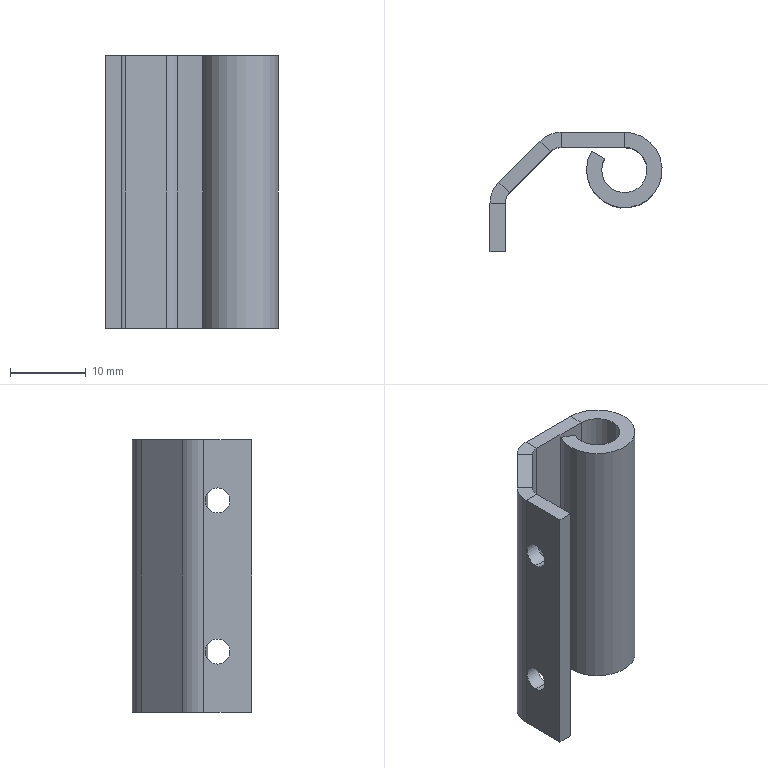Part | SolidWorks | features EdgeFlange 2, FlatPattern 1, Hem 1, HoleWzd 1, SMBaseFlange 1, SheetMetal 1 | 1 solid | 30 faces | box 22.778 x 15.778 x 36 mm | volume 3424 mm3 | plane 20 | cylinder 10 | commonest cylinder face diameters 3.3 x4 4 x2 8 x2 6 x1 10 x1
STEP:
#1=CARTESIAN_POINT('',(-12.278,-11.278,-11.65));
#2=VERTEX_POINT('',#1);
#3=CARTESIAN_POINT('',(-12.278,-11.278,-8.35));
#4=VERTEX_POINT('',#3);
#5=CARTESIAN_POINT('',(-12.278,-11.278,-10.));
#6=DIRECTION('',(-1.,0.,0.));
#7=DIRECTION('',(0.,-1.,0.));
#8=AXIS2_PLACEMENT_3D('',#5,#6,#7);
#9=CIRCLE('',#8,1.65);
#10=EDGE_CURVE('',#2,#4,#9,.T.);
#11=ORIENTED_EDGE('',*,*,#10,.F.);
#12=CARTESIAN_POINT('',(-14.278,-11.278,-11.65));
#13=VERTEX_POINT('',#12);
#14=CARTESIAN_POINT('',(-14.278,-11.278,-11.65));
#15=DIRECTION('',(-1.,0.,0.));
#16=VECTOR('',#15,1000.);
#17=LINE('',#14,#16);
#18=EDGE_CURVE('',#2,#13,#17,.T.);
#19=ORIENTED_EDGE('',*,*,#18,.T.);
#20=CARTESIAN_POINT('',(-14.278,-11.278,-8.35));
#21=VERTEX_POINT('',#20);
#22=CARTESIAN_POINT('',(-14.278,-11.278,-10.));
#23=DIRECTION('',(-1.,0.,0.));
#24=DIRECTION('',(0.,0.,1.));
#25=AXIS2_PLACEMENT_3D('',#22,#23,#24);
#26=CIRCLE('',#25,1.65);
#27=EDGE_CURVE('',#13,#21,#26,.T.);
#28=ORIENTED_EDGE('',*,*,#27,.T.);
#29=CARTESIAN_POINT('',(-14.278,-11.278,-8.35));
#30=DIRECTION('',(-1.,0.,0.));
#31=VECTOR('',#30,1000.);
#32=LINE('',#29,#31);
#33=EDGE_CURVE('',#4,#21,#32,.T.);
#34=ORIENTED_EDGE('',*,*,#33,.F.);
#35=EDGE_LOOP('',(#11,#19,#28,#34));
#36=FACE_OUTER_BOUND('',#35,.T.);
#37=CARTESIAN_POINT('',(-14.278,-11.278,-10.));
#38=DIRECTION('',(-1.,0.,0.));
#39=DIRECTION('',(0.,0.,1.));
#40=AXIS2_PLACEMENT_3D('',#37,#38,#39);
#41=CYLINDRICAL_SURFACE('',#40,1.65);
#42=ADVANCED_FACE('',(#36),#41,.F.);
#43=CARTESIAN_POINT('',(-12.278,-11.278,8.35));
#44=VERTEX_POINT('',#43);
#45=CARTESIAN_POINT('',(-12.278,-11.278,11.65));
#46=VERTEX_POINT('',#45);
#47=CARTESIAN_POINT('',(-12.278,-11.278,10.));
#48=DIRECTION('',(-1.,0.,0.));
#49=DIRECTION('',(0.,-1.,0.));
#50=AXIS2_PLACEMENT_3D('',#47,#48,#49);
#51=CIRCLE('',#50,1.65);
#52=EDGE_CURVE('',#44,#46,#51,.T.);
#53=ORIENTED_EDGE('',*,*,#52,.F.);
#54=CARTESIAN_POINT('',(-14.278,-11.278,8.35));
#55=VERTEX_POINT('',#54);
#56=CARTESIAN_POINT('',(-14.278,-11.278,8.35));
#57=DIRECTION('',(-1.,0.,0.));
#58=VECTOR('',#57,1000.);
#59=LINE('',#56,#58);
#60=EDGE_CURVE('',#44,#55,#59,.T.);
#61=ORIENTED_EDGE('',*,*,#60,.T.);
#62=CARTESIAN_POINT('',(-14.278,-11.278,11.65));
#63=VERTEX_POINT('',#62);
#64=CARTESIAN_POINT('',(-14.278,-11.278,10.));
#65=DIRECTION('',(-1.,0.,0.));
#66=DIRECTION('',(0.,0.,1.));
#67=AXIS2_PLACEMENT_3D('',#64,#65,#66);
#68=CIRCLE('',#67,1.65);
#69=EDGE_CURVE('',#55,#63,#68,.T.);
#70=ORIENTED_EDGE('',*,*,#69,.T.);
#71=CARTESIAN_POINT('',(-14.278,-11.278,11.65));
#72=DIRECTION('',(-1.,0.,0.));
#73=VECTOR('',#72,1000.);
#74=LINE('',#71,#73);
#75=EDGE_CURVE('',#46,#63,#74,.T.);
#76=ORIENTED_EDGE('',*,*,#75,.F.);
#77=EDGE_LOOP('',(#53,#61,#70,#76));
#78=FACE_OUTER_BOUND('',#77,.T.);
#79=CARTESIAN_POINT('',(-14.278,-11.278,10.));
#80=DIRECTION('',(-1.,0.,0.));
#81=DIRECTION('',(0.,0.,1.));
#82=AXIS2_PLACEMENT_3D('',#79,#80,#81);
#83=CYLINDRICAL_SURFACE('',#82,1.65);
#84=ADVANCED_FACE('',(#78),#83,.F.);
#85=CARTESIAN_POINT('',(-11.692,-8.021,-18.));
#86=VERTEX_POINT('',#85);
#87=CARTESIAN_POINT('',(-6.257,-2.586,-18.));
#88=VERTEX_POINT('',#87);
#89=CARTESIAN_POINT('',(-0.4216,3.25,-18.));
#90=DIRECTION('',(0.7071,0.7071,0.));
#91=VECTOR('',#90,1000.);
#92=LINE('',#89,#91);
#93=EDGE_CURVE('',#86,#88,#92,.T.);
#94=ORIENTED_EDGE('',*,*,#93,.F.);
#95=CARTESIAN_POINT('',(-13.107,-6.607,-18.));
#96=VERTEX_POINT('',#95);
#97=CARTESIAN_POINT('',(-11.692,-8.021,-18.));
#98=DIRECTION('',(-0.7071,0.7071,0.));
#99=VECTOR('',#98,1000.);
#100=LINE('',#97,#99);
#101=EDGE_CURVE('',#86,#96,#100,.T.);
#102=ORIENTED_EDGE('',*,*,#101,.T.);
#103=CARTESIAN_POINT('',(-7.672,-1.172,-18.));
#104=VERTEX_POINT('',#103);
#105=CARTESIAN_POINT('',(-7.086,-0.5858,-18.));
#106=DIRECTION('',(0.7071,0.7071,0.));
#107=VECTOR('',#106,1000.);
#108=LINE('',#105,#107);
#109=EDGE_CURVE('',#96,#104,#108,.T.);
#110=ORIENTED_EDGE('',*,*,#109,.T.);
#111=CARTESIAN_POINT('',(-6.257,-2.586,-18.));
#112=DIRECTION('',(-0.7071,0.7071,0.));
#113=VECTOR('',#112,1000.);
#114=LINE('',#111,#113);
#115=EDGE_CURVE('',#88,#104,#114,.T.);
#116=ORIENTED_EDGE('',*,*,#115,.F.);
#117=EDGE_LOOP('',(#94,#102,#110,#116));
#118=FACE_OUTER_BOUND('',#117,.T.);
#119=CARTESIAN_POINT('',(-7.086,-0.5858,-18.));
#120=DIRECTION('',(0.,0.,-1.));
#121=DIRECTION('',(-1.,0.,0.));
#122=AXIS2_PLACEMENT_3D('',#119,#120,#121);
#123=PLANE('',#122);
#124=ADVANCED_FACE('',(#118),#123,.T.);
#125=ORIENTED_EDGE('',*,*,#109,.F.);
#126=CARTESIAN_POINT('',(-13.107,-6.607,18.));
#127=VERTEX_POINT('',#126);
#128=CARTESIAN_POINT('',(-13.107,-6.607,-18.));
#129=DIRECTION('',(0.,0.,1.));
#130=VECTOR('',#129,1000.);
#131=LINE('',#128,#130);
#132=EDGE_CURVE('',#96,#127,#131,.T.);
#133=ORIENTED_EDGE('',*,*,#132,.T.);
#134=CARTESIAN_POINT('',(-7.672,-1.172,18.));
#135=VERTEX_POINT('',#134);
#136=CARTESIAN_POINT('',(-15.692,-9.192,18.));
#137=DIRECTION('',(-0.7071,-0.7071,0.));
#138=VECTOR('',#137,1000.);
#139=LINE('',#136,#138);
#140=EDGE_CURVE('',#135,#127,#139,.T.);
#141=ORIENTED_EDGE('',*,*,#140,.F.);
#142=CARTESIAN_POINT('',(-7.672,-1.172,0.));
#143=DIRECTION('',(0.,0.,-1.));
#144=VECTOR('',#143,1000.);
#145=LINE('',#142,#144);
#146=EDGE_CURVE('',#135,#104,#145,.T.);
#147=ORIENTED_EDGE('',*,*,#146,.T.);
#148=EDGE_LOOP('',(#125,#133,#141,#147));
#149=FACE_OUTER_BOUND('',#148,.T.);
#150=CARTESIAN_POINT('',(-1.836,4.664,0.));
#151=DIRECTION('',(-0.7071,0.7071,0.));
#152=DIRECTION('',(-0.7071,-0.7071,0.));
#153=AXIS2_PLACEMENT_3D('',#150,#151,#152);
#154=PLANE('',#153);
#155=ADVANCED_FACE('',(#149),#154,.T.);
#156=CARTESIAN_POINT('',(-11.692,-8.021,18.));
#157=VERTEX_POINT('',#156);
#158=CARTESIAN_POINT('',(-11.692,-8.021,-18.));
#159=DIRECTION('',(0.,0.,1.));
#160=VECTOR('',#159,1000.);
#161=LINE('',#158,#160);
#162=EDGE_CURVE('',#86,#157,#161,.T.);
#163=ORIENTED_EDGE('',*,*,#162,.F.);
#164=ORIENTED_EDGE('',*,*,#93,.T.);
#165=CARTESIAN_POINT('',(-6.257,-2.586,18.));
#166=VERTEX_POINT('',#165);
#167=CARTESIAN_POINT('',(-6.257,-2.586,18.));
#168=DIRECTION('',(0.,0.,-1.));
#169=VECTOR('',#168,1000.);
#170=LINE('',#167,#169);
#171=EDGE_CURVE('',#166,#88,#170,.T.);
#172=ORIENTED_EDGE('',*,*,#171,.F.);
#173=CARTESIAN_POINT('',(-0.4216,3.25,18.));
#174=DIRECTION('',(-0.7071,-0.7071,0.));
#175=VECTOR('',#174,1000.);
#176=LINE('',#173,#175);
#177=EDGE_CURVE('',#166,#157,#176,.T.);
#178=ORIENTED_EDGE('',*,*,#177,.T.);
#179=EDGE_LOOP('',(#163,#164,#172,#178));
#180=FACE_OUTER_BOUND('',#179,.T.);
#181=CARTESIAN_POINT('',(-0.4216,3.25,0.));
#182=DIRECTION('',(-0.7071,0.7071,0.));
#183=DIRECTION('',(-0.7071,-0.7071,0.));
#184=AXIS2_PLACEMENT_3D('',#181,#182,#183);
#185=PLANE('',#184);
#186=ADVANCED_FACE('',(#180),#185,.F.);
#187=CARTESIAN_POINT('',(3.5,-2.,-18.));
#188=VERTEX_POINT('',#187);
#189=CARTESIAN_POINT('',(-4.843,-2.,-18.));
#190=VERTEX_POINT('',#189);
#191=CARTESIAN_POINT('',(-8.5,-2.,-18.));
#192=DIRECTION('',(-1.,0.,0.));
#193=VECTOR('',#192,1000.);
#194=LINE('',#191,#193);
#195=EDGE_CURVE('',#188,#190,#194,.T.);
#196=ORIENTED_EDGE('',*,*,#195,.T.);
#197=CARTESIAN_POINT('',(-4.843,0.,-18.));
#198=VERTEX_POINT('',#197);
#199=CARTESIAN_POINT('',(-4.843,-2.,-18.));
#200=DIRECTION('',(0.,1.,0.));
#201=VECTOR('',#200,1000.);
#202=LINE('',#199,#201);
#203=EDGE_CURVE('',#190,#198,#202,.T.);
#204=ORIENTED_EDGE('',*,*,#203,.T.);
#205=CARTESIAN_POINT('',(3.5,0.,-18.));
#206=VERTEX_POINT('',#205);
#207=CARTESIAN_POINT('',(-8.5,0.,-18.));
#208=DIRECTION('',(-1.,0.,0.));
#209=VECTOR('',#208,1000.);
#210=LINE('',#207,#209);
#211=EDGE_CURVE('',#206,#198,#210,.T.);
#212=ORIENTED_EDGE('',*,*,#211,.F.);
#213=CARTESIAN_POINT('',(3.5,-2.,-18.));
#214=DIRECTION('',(0.,1.,0.));
#215=VECTOR('',#214,1000.);
#216=LINE('',#213,#215);
#217=EDGE_CURVE('',#188,#206,#216,.T.);
#218=ORIENTED_EDGE('',*,*,#217,.F.);
#219=EDGE_LOOP('',(#196,#204,#212,#218));
#220=FACE_OUTER_BOUND('',#219,.T.);
#221=CARTESIAN_POINT('',(-8.5,-2.,-18.));
#222=DIRECTION('',(0.,0.,-1.));
#223=DIRECTION('',(-1.,0.,0.));
#224=AXIS2_PLACEMENT_3D('',#221,#222,#223);
#225=PLANE('',#224);
#226=ADVANCED_FACE('',(#220),#225,.T.);
#227=CARTESIAN_POINT('',(-4.843,-2.,18.));
#228=VERTEX_POINT('',#227);
#229=CARTESIAN_POINT('',(-4.843,-2.,-18.));
#230=DIRECTION('',(0.,0.,1.));
#231=VECTOR('',#230,1000.);
#232=LINE('',#229,#231);
#233=EDGE_CURVE('',#190,#228,#232,.T.);
#234=ORIENTED_EDGE('',*,*,#233,.F.);
#235=ORIENTED_EDGE('',*,*,#195,.F.);
#236=CARTESIAN_POINT('',(3.5,-2.,18.));
#237=VERTEX_POINT('',#236);
#238=CARTESIAN_POINT('',(3.5,-2.,18.));
#239=DIRECTION('',(0.,0.,-1.));
#240=VECTOR('',#239,1000.);
#241=LINE('',#238,#240);
#242=EDGE_CURVE('',#237,#188,#241,.T.);
#243=ORIENTED_EDGE('',*,*,#242,.F.);
#244=CARTESIAN_POINT('',(-8.5,-2.,18.));
#245=DIRECTION('',(1.,0.,0.));
#246=VECTOR('',#245,1000.);
#247=LINE('',#244,#246);
#248=EDGE_CURVE('',#228,#237,#247,.T.);
#249=ORIENTED_EDGE('',*,*,#248,.F.);
#250=EDGE_LOOP('',(#234,#235,#243,#249));
#251=FACE_OUTER_BOUND('',#250,.T.);
#252=CARTESIAN_POINT('',(0.,-2.,0.));
#253=DIRECTION('',(0.,1.,0.));
#254=DIRECTION('',(0.,0.,1.));
#255=AXIS2_PLACEMENT_3D('',#252,#253,#254);
#256=PLANE('',#255);
#257=ADVANCED_FACE('',(#251),#256,.F.);
#258=ORIENTED_EDGE('',*,*,#211,.T.);
#259=CARTESIAN_POINT('',(-4.843,0.,18.));
#260=VERTEX_POINT('',#259);
#261=CARTESIAN_POINT('',(-4.843,0.,-18.));
#262=DIRECTION('',(0.,0.,1.));
#263=VECTOR('',#262,1000.);
#264=LINE('',#261,#263);
#265=EDGE_CURVE('',#198,#260,#264,.T.);
#266=ORIENTED_EDGE('',*,*,#265,.T.);
#267=CARTESIAN_POINT('',(3.5,0.,18.));
#268=VERTEX_POINT('',#267);
#269=CARTESIAN_POINT('',(-8.5,0.,18.));
#270=DIRECTION('',(1.,0.,0.));
#271=VECTOR('',#270,1000.);
#272=LINE('',#269,#271);
#273=EDGE_CURVE('',#260,#268,#272,.T.);
#274=ORIENTED_EDGE('',*,*,#273,.T.);
#275=CARTESIAN_POINT('',(3.5,0.,18.));
#276=DIRECTION('',(0.,0.,-1.));
#277=VECTOR('',#276,1000.);
#278=LINE('',#275,#277);
#279=EDGE_CURVE('',#268,#206,#278,.T.);
#280=ORIENTED_EDGE('',*,*,#279,.T.);
#281=EDGE_LOOP('',(#258,#266,#274,#280));
#282=FACE_OUTER_BOUND('',#281,.T.);
#283=CARTESIAN_POINT('',(0.,0.,0.));
#284=DIRECTION('',(0.,1.,0.));
#285=DIRECTION('',(0.,0.,1.));
#286=AXIS2_PLACEMENT_3D('',#283,#284,#285);
#287=PLANE('',#286);
#288=ADVANCED_FACE('',(#282),#287,.T.);
#289=CARTESIAN_POINT('',(-4.843,-2.,18.));
#290=DIRECTION('',(0.,1.,0.));
#291=VECTOR('',#290,1000.);
#292=LINE('',#289,#291);
#293=EDGE_CURVE('',#228,#260,#292,.T.);
#294=ORIENTED_EDGE('',*,*,#293,.F.);
#295=ORIENTED_EDGE('',*,*,#248,.T.);
#296=CARTESIAN_POINT('',(3.5,-2.,18.));
#297=DIRECTION('',(0.,1.,0.));
#298=VECTOR('',#297,1000.);
#299=LINE('',#296,#298);
#300=EDGE_CURVE('',#237,#268,#299,.T.);
#301=ORIENTED_EDGE('',*,*,#300,.T.);
#302=ORIENTED_EDGE('',*,*,#273,.F.);
#303=EDGE_LOOP('',(#294,#295,#301,#302));
#304=FACE_OUTER_BOUND('',#303,.T.);
#305=CARTESIAN_POINT('',(-8.5,-2.,18.));
#306=DIRECTION('',(0.,0.,1.));
#307=DIRECTION('',(1.,0.,0.));
#308=AXIS2_PLACEMENT_3D('',#305,#306,#307);
#309=PLANE('',#308);
#310=ADVANCED_FACE('',(#304),#309,.T.);
#311=CARTESIAN_POINT('',(0.9019,-3.5,18.));
#312=VERTEX_POINT('',#311);
#313=CARTESIAN_POINT('',(-0.8301,-2.5,18.));
#314=VERTEX_POINT('',#313);
#315=CARTESIAN_POINT('',(0.9019,-3.5,18.));
#316=DIRECTION('',(-0.866,0.5,0.));
#317=VECTOR('',#316,1000.);
#318=LINE('',#315,#317);
#319=EDGE_CURVE('',#312,#314,#318,.T.);
#320=ORIENTED_EDGE('',*,*,#319,.F.);
#321=CARTESIAN_POINT('',(0.9019,-3.5,-18.));
#322=VERTEX_POINT('',#321);
#323=CARTESIAN_POINT('',(0.9019,-3.5,18.));
#324=DIRECTION('',(0.,0.,1.));
#325=VECTOR('',#324,1000.);
#326=LINE('',#323,#325);
#327=EDGE_CURVE('',#322,#312,#326,.T.);
#328=ORIENTED_EDGE('',*,*,#327,.F.);
#329=CARTESIAN_POINT('',(-0.8301,-2.5,-18.));
#330=VERTEX_POINT('',#329);
#331=CARTESIAN_POINT('',(0.9019,-3.5,-18.));
#332=DIRECTION('',(-0.866,0.5,0.));
#333=VECTOR('',#332,1000.);
#334=LINE('',#331,#333);
#335=EDGE_CURVE('',#322,#330,#334,.T.);
#336=ORIENTED_EDGE('',*,*,#335,.T.);
#337=CARTESIAN_POINT('',(-0.8301,-2.5,18.));
#338=DIRECTION('',(0.,0.,1.));
#339=VECTOR('',#338,1000.);
#340=LINE('',#337,#339);
#341=EDGE_CURVE('',#330,#314,#340,.T.);
#342=ORIENTED_EDGE('',*,*,#341,.T.);
#343=EDGE_LOOP('',(#320,#328,#336,#342));
#344=FACE_OUTER_BOUND('',#343,.T.);
#345=CARTESIAN_POINT('',(0.9019,-3.5,0.));
#346=DIRECTION('',(-0.5,-0.866,0.));
#347=DIRECTION('',(0.,0.,1.));
#348=AXIS2_PLACEMENT_3D('',#345,#346,#347);
#349=PLANE('',#348);
#350=ADVANCED_FACE('',(#344),#349,.F.);
#351=ORIENTED_EDGE('',*,*,#335,.F.);
#352=CARTESIAN_POINT('',(3.5,-5.,-18.));
#353=DIRECTION('',(0.,0.,-1.));
#354=DIRECTION('',(1.,0.,0.));
#355=AXIS2_PLACEMENT_3D('',#352,#353,#354);
#356=CIRCLE('',#355,3.);
#357=EDGE_CURVE('',#188,#322,#356,.T.);
#358=ORIENTED_EDGE('',*,*,#357,.F.);
#359=ORIENTED_EDGE('',*,*,#217,.T.);
#360=CARTESIAN_POINT('',(3.5,-5.,-18.));
#361=DIRECTION('',(0.,0.,-1.));
#362=DIRECTION('',(1.,0.,0.));
#363=AXIS2_PLACEMENT_3D('',#360,#361,#362);
#364=CIRCLE('',#363,5.);
#365=EDGE_CURVE('',#206,#330,#364,.T.);
#366=ORIENTED_EDGE('',*,*,#365,.T.);
#367=EDGE_LOOP('',(#351,#358,#359,#366));
#368=FACE_OUTER_BOUND('',#367,.T.);
#369=CARTESIAN_POINT('',(3.5,-5.,-18.));
#370=DIRECTION('',(0.,0.,-1.));
#371=DIRECTION('',(-1.,0.,0.));
#372=AXIS2_PLACEMENT_3D('',#369,#370,#371);
#373=PLANE('',#372);
#374=ADVANCED_FACE('',(#368),#373,.T.);
#375=CARTESIAN_POINT('',(3.5,-5.,18.));
#376=DIRECTION('',(0.,0.,1.));
#377=DIRECTION('',(1.,0.,0.));
#378=AXIS2_PLACEMENT_3D('',#375,#376,#377);
#379=CIRCLE('',#378,3.);
#380=EDGE_CURVE('',#312,#237,#379,.T.);
#381=ORIENTED_EDGE('',*,*,#380,.F.);
#382=ORIENTED_EDGE('',*,*,#319,.T.);
#383=CARTESIAN_POINT('',(3.5,-5.,18.));
#384=DIRECTION('',(0.,0.,1.));
#385=DIRECTION('',(1.,0.,0.));
#386=AXIS2_PLACEMENT_3D('',#383,#384,#385);
#387=CIRCLE('',#386,5.);
#388=EDGE_CURVE('',#314,#268,#387,.T.);
#389=ORIENTED_EDGE('',*,*,#388,.T.);
#390=ORIENTED_EDGE('',*,*,#300,.F.);
#391=EDGE_LOOP('',(#381,#382,#389,#390));
#392=FACE_OUTER_BOUND('',#391,.T.);
#393=CARTESIAN_POINT('',(3.5,-5.,18.));
#394=DIRECTION('',(0.,0.,-1.));
#395=DIRECTION('',(-1.,0.,0.));
#396=AXIS2_PLACEMENT_3D('',#393,#394,#395);
#397=PLANE('',#396);
#398=ADVANCED_FACE('',(#392),#397,.F.);
#399=ORIENTED_EDGE('',*,*,#279,.F.);
#400=ORIENTED_EDGE('',*,*,#388,.F.);
#401=ORIENTED_EDGE('',*,*,#341,.F.);
#402=ORIENTED_EDGE('',*,*,#365,.F.);
#403=EDGE_LOOP('',(#399,#400,#401,#402));
#404=FACE_OUTER_BOUND('',#403,.T.);
#405=CARTESIAN_POINT('',(3.5,-5.,18.));
#406=DIRECTION('',(0.,0.,1.));
#407=DIRECTION('',(-0.866,0.5,0.));
#408=AXIS2_PLACEMENT_3D('',#405,#406,#407);
#409=CYLINDRICAL_SURFACE('',#408,5.);
#410=ADVANCED_FACE('',(#404),#409,.T.);
#411=ORIENTED_EDGE('',*,*,#242,.T.);
#412=ORIENTED_EDGE('',*,*,#357,.T.);
#413=ORIENTED_EDGE('',*,*,#327,.T.);
#414=ORIENTED_EDGE('',*,*,#380,.T.);
#415=EDGE_LOOP('',(#411,#412,#413,#414));
#416=FACE_OUTER_BOUND('',#415,.T.);
#417=CARTESIAN_POINT('',(3.5,-5.,18.));
#418=DIRECTION('',(0.,0.,1.));
#419=DIRECTION('',(-0.866,0.5,0.));
#420=AXIS2_PLACEMENT_3D('',#417,#418,#419);
#421=CYLINDRICAL_SURFACE('',#420,3.);
#422=ADVANCED_FACE('',(#416),#421,.F.);
#423=CARTESIAN_POINT('',(-7.672,-1.172,18.));
#424=DIRECTION('',(-0.7071,0.7071,0.));
#425=VECTOR('',#424,1000.);
#426=LINE('',#423,#425);
#427=EDGE_CURVE('',#166,#135,#426,.T.);
#428=ORIENTED_EDGE('',*,*,#427,.F.);
#429=CARTESIAN_POINT('',(-4.843,-4.,18.));
#430=DIRECTION('',(0.,0.,1.));
#431=DIRECTION('',(-1.,0.,0.));
#432=AXIS2_PLACEMENT_3D('',#429,#430,#431);
#433=CIRCLE('',#432,2.);
#434=EDGE_CURVE('',#228,#166,#433,.T.);
#435=ORIENTED_EDGE('',*,*,#434,.F.);
#436=ORIENTED_EDGE('',*,*,#293,.T.);
#437=CARTESIAN_POINT('',(-4.843,-4.,18.));
#438=DIRECTION('',(0.,0.,1.));
#439=DIRECTION('',(-1.,0.,0.));
#440=AXIS2_PLACEMENT_3D('',#437,#438,#439);
#441=CIRCLE('',#440,4.);
#442=EDGE_CURVE('',#260,#135,#441,.T.);
#443=ORIENTED_EDGE('',*,*,#442,.T.);
#444=EDGE_LOOP('',(#428,#435,#436,#443));
#445=FACE_OUTER_BOUND('',#444,.T.);
#446=CARTESIAN_POINT('',(-4.843,-4.,18.));
#447=DIRECTION('',(0.,0.,1.));
#448=DIRECTION('',(1.,0.,0.));
#449=AXIS2_PLACEMENT_3D('',#446,#447,#448);
#450=PLANE('',#449);
#451=ADVANCED_FACE('',(#445),#450,.T.);
#452=CARTESIAN_POINT('',(-4.843,-4.,-18.));
#453=DIRECTION('',(0.,0.,-1.));
#454=DIRECTION('',(-1.,0.,0.));
#455=AXIS2_PLACEMENT_3D('',#452,#453,#454);
#456=CIRCLE('',#455,2.);
#457=EDGE_CURVE('',#88,#190,#456,.T.);
#458=ORIENTED_EDGE('',*,*,#457,.F.);
#459=ORIENTED_EDGE('',*,*,#115,.T.);
#460=CARTESIAN_POINT('',(-4.843,-4.,-18.));
#461=DIRECTION('',(0.,0.,-1.));
#462=DIRECTION('',(-1.,0.,0.));
#463=AXIS2_PLACEMENT_3D('',#460,#461,#462);
#464=CIRCLE('',#463,4.);
#465=EDGE_CURVE('',#104,#198,#464,.T.);
#466=ORIENTED_EDGE('',*,*,#465,.T.);
#467=ORIENTED_EDGE('',*,*,#203,.F.);
#468=EDGE_LOOP('',(#458,#459,#466,#467));
#469=FACE_OUTER_BOUND('',#468,.T.);
#470=CARTESIAN_POINT('',(-4.843,-4.,-18.));
#471=DIRECTION('',(0.,0.,1.));
#472=DIRECTION('',(1.,0.,0.));
#473=AXIS2_PLACEMENT_3D('',#470,#471,#472);
#474=PLANE('',#473);
#475=ADVANCED_FACE('',(#469),#474,.F.);
#476=ORIENTED_EDGE('',*,*,#265,.F.);
#477=ORIENTED_EDGE('',*,*,#465,.F.);
#478=ORIENTED_EDGE('',*,*,#146,.F.);
#479=ORIENTED_EDGE('',*,*,#442,.F.);
#480=EDGE_LOOP('',(#476,#477,#478,#479));
#481=FACE_OUTER_BOUND('',#480,.T.);
#482=CARTESIAN_POINT('',(-4.843,-4.,-18.));
#483=DIRECTION('',(0.,0.,-1.));
#484=DIRECTION('',(-0.7071,0.7071,0.));
#485=AXIS2_PLACEMENT_3D('',#482,#483,#484);
#486=CYLINDRICAL_SURFACE('',#485,4.);
#487=ADVANCED_FACE('',(#481),#486,.T.);
#488=ORIENTED_EDGE('',*,*,#233,.T.);
#489=ORIENTED_EDGE('',*,*,#434,.T.);
#490=ORIENTED_EDGE('',*,*,#171,.T.);
#491=ORIENTED_EDGE('',*,*,#457,.T.);
#492=EDGE_LOOP('',(#488,#489,#490,#491));
#493=FACE_OUTER_BOUND('',#492,.T.);
#494=CARTESIAN_POINT('',(-4.843,-4.,-18.));
#495=DIRECTION('',(0.,0.,-1.));
#496=DIRECTION('',(-0.7071,0.7071,0.));
#497=AXIS2_PLACEMENT_3D('',#494,#495,#496);
#498=CYLINDRICAL_SURFACE('',#497,2.);
#499=ADVANCED_FACE('',(#493),#498,.F.);
#500=CARTESIAN_POINT('',(-11.692,-8.021,18.));
#501=DIRECTION('',(-0.7071,0.7071,0.));
#502=VECTOR('',#501,1000.);
#503=LINE('',#500,#502);
#504=EDGE_CURVE('',#157,#127,#503,.T.);
#505=ORIENTED_EDGE('',*,*,#504,.F.);
#506=ORIENTED_EDGE('',*,*,#177,.F.);
#507=ORIENTED_EDGE('',*,*,#427,.T.);
#508=ORIENTED_EDGE('',*,*,#140,.T.);
#509=EDGE_LOOP('',(#505,#506,#507,#508));
#510=FACE_OUTER_BOUND('',#509,.T.);
#511=CARTESIAN_POINT('',(-15.692,-9.192,18.));
#512=DIRECTION('',(0.,0.,1.));
#513=DIRECTION('',(1.,0.,0.));
#514=AXIS2_PLACEMENT_3D('',#511,#512,#513);
#515=PLANE('',#514);
#516=ADVANCED_FACE('',(#510),#515,.T.);
#517=CARTESIAN_POINT('',(-12.278,-9.435,18.));
#518=VERTEX_POINT('',#517);
#519=CARTESIAN_POINT('',(-14.278,-9.435,18.));
#520=VERTEX_POINT('',#519);
#521=CARTESIAN_POINT('',(-14.278,-9.435,18.));
#522=DIRECTION('',(-1.,0.,0.));
#523=VECTOR('',#522,1000.);
#524=LINE('',#521,#523);
#525=EDGE_CURVE('',#518,#520,#524,.T.);
#526=ORIENTED_EDGE('',*,*,#525,.F.);
#527=CARTESIAN_POINT('',(-10.278,-9.435,18.));
#528=DIRECTION('',(0.,0.,1.));
#529=DIRECTION('',(-1.,0.,0.));
#530=AXIS2_PLACEMENT_3D('',#527,#528,#529);
#531=CIRCLE('',#530,2.);
#532=EDGE_CURVE('',#157,#518,#531,.T.);
#533=ORIENTED_EDGE('',*,*,#532,.F.);
#534=ORIENTED_EDGE('',*,*,#504,.T.);
#535=CARTESIAN_POINT('',(-10.278,-9.435,18.));
#536=DIRECTION('',(0.,0.,1.));
#537=DIRECTION('',(-1.,0.,0.));
#538=AXIS2_PLACEMENT_3D('',#535,#536,#537);
#539=CIRCLE('',#538,4.);
#540=EDGE_CURVE('',#127,#520,#539,.T.);
#541=ORIENTED_EDGE('',*,*,#540,.T.);
#542=EDGE_LOOP('',(#526,#533,#534,#541));
#543=FACE_OUTER_BOUND('',#542,.T.);
#544=CARTESIAN_POINT('',(-10.278,-9.435,18.));
#545=DIRECTION('',(0.,0.,1.));
#546=DIRECTION('',(1.,0.,0.));
#547=AXIS2_PLACEMENT_3D('',#544,#545,#546);
#548=PLANE('',#547);
#549=ADVANCED_FACE('',(#543),#548,.T.);
#550=CARTESIAN_POINT('',(-12.278,-9.435,-18.));
#551=VERTEX_POINT('',#550);
#552=CARTESIAN_POINT('',(-10.278,-9.435,-18.));
#553=DIRECTION('',(0.,0.,-1.));
#554=DIRECTION('',(-1.,0.,0.));
#555=AXIS2_PLACEMENT_3D('',#552,#553,#554);
#556=CIRCLE('',#555,2.);
#557=EDGE_CURVE('',#551,#86,#556,.T.);
#558=ORIENTED_EDGE('',*,*,#557,.F.);
#559=CARTESIAN_POINT('',(-14.278,-9.435,-18.));
#560=VERTEX_POINT('',#559);
#561=CARTESIAN_POINT('',(-12.278,-9.435,-18.));
#562=DIRECTION('',(-1.,0.,0.));
#563=VECTOR('',#562,1000.);
#564=LINE('',#561,#563);
#565=EDGE_CURVE('',#551,#560,#564,.T.);
#566=ORIENTED_EDGE('',*,*,#565,.T.);
#567=CARTESIAN_POINT('',(-10.278,-9.435,-18.));
#568=DIRECTION('',(0.,0.,-1.));
#569=DIRECTION('',(-1.,0.,0.));
#570=AXIS2_PLACEMENT_3D('',#567,#568,#569);
#571=CIRCLE('',#570,4.);
#572=EDGE_CURVE('',#560,#96,#571,.T.);
#573=ORIENTED_EDGE('',*,*,#572,.T.);
#574=ORIENTED_EDGE('',*,*,#101,.F.);
#575=EDGE_LOOP('',(#558,#566,#573,#574));
#576=FACE_OUTER_BOUND('',#575,.T.);
#577=CARTESIAN_POINT('',(-10.278,-9.435,-18.));
#578=DIRECTION('',(0.,0.,1.));
#579=DIRECTION('',(1.,0.,0.));
#580=AXIS2_PLACEMENT_3D('',#577,#578,#579);
#581=PLANE('',#580);
#582=ADVANCED_FACE('',(#576),#581,.F.);
#583=ORIENTED_EDGE('',*,*,#132,.F.);
#584=ORIENTED_EDGE('',*,*,#572,.F.);
#585=CARTESIAN_POINT('',(-14.278,-9.435,0.));
#586=DIRECTION('',(0.,0.,-1.));
#587=VECTOR('',#586,1000.);
#588=LINE('',#585,#587);
#589=EDGE_CURVE('',#520,#560,#588,.T.);
#590=ORIENTED_EDGE('',*,*,#589,.F.);
#591=ORIENTED_EDGE('',*,*,#540,.F.);
#592=EDGE_LOOP('',(#583,#584,#590,#591));
#593=FACE_OUTER_BOUND('',#592,.T.);
#594=CARTESIAN_POINT('',(-10.278,-9.435,-18.));
#595=DIRECTION('',(0.,0.,-1.));
#596=DIRECTION('',(-1.,0.,0.));
#597=AXIS2_PLACEMENT_3D('',#594,#595,#596);
#598=CYLINDRICAL_SURFACE('',#597,4.);
#599=ADVANCED_FACE('',(#593),#598,.T.);
#600=ORIENTED_EDGE('',*,*,#162,.T.);
#601=ORIENTED_EDGE('',*,*,#532,.T.);
#602=CARTESIAN_POINT('',(-12.278,-9.435,18.));
#603=DIRECTION('',(0.,0.,-1.));
#604=VECTOR('',#603,1000.);
#605=LINE('',#602,#604);
#606=EDGE_CURVE('',#518,#551,#605,.T.);
#607=ORIENTED_EDGE('',*,*,#606,.T.);
#608=ORIENTED_EDGE('',*,*,#557,.T.);
#609=EDGE_LOOP('',(#600,#601,#607,#608));
#610=FACE_OUTER_BOUND('',#609,.T.);
#611=CARTESIAN_POINT('',(-10.278,-9.435,-18.));
#612=DIRECTION('',(0.,0.,-1.));
#613=DIRECTION('',(-1.,0.,0.));
#614=AXIS2_PLACEMENT_3D('',#611,#612,#613);
#615=CYLINDRICAL_SURFACE('',#614,2.);
#616=ADVANCED_FACE('',(#610),#615,.F.);
#617=CARTESIAN_POINT('',(-14.278,-15.778,-18.));
#618=VERTEX_POINT('',#617);
#619=CARTESIAN_POINT('',(-14.278,-8.607,-18.));
#620=DIRECTION('',(0.,1.,0.));
#621=VECTOR('',#620,1000.);
#622=LINE('',#619,#621);
#623=EDGE_CURVE('',#618,#560,#622,.T.);
#624=ORIENTED_EDGE('',*,*,#623,.T.);
#625=ORIENTED_EDGE('',*,*,#565,.F.);
#626=CARTESIAN_POINT('',(-12.278,-15.778,-18.));
#627=VERTEX_POINT('',#626);
#628=CARTESIAN_POINT('',(-12.278,2.,-18.));
#629=DIRECTION('',(0.,1.,0.));
#630=VECTOR('',#629,1000.);
#631=LINE('',#628,#630);
#632=EDGE_CURVE('',#627,#551,#631,.T.);
#633=ORIENTED_EDGE('',*,*,#632,.F.);
#634=CARTESIAN_POINT('',(-14.278,-15.778,-18.));
#635=DIRECTION('',(1.,0.,0.));
#636=VECTOR('',#635,1000.);
#637=LINE('',#634,#636);
#638=EDGE_CURVE('',#618,#627,#637,.T.);
#639=ORIENTED_EDGE('',*,*,#638,.F.);
#640=EDGE_LOOP('',(#624,#625,#633,#639));
#641=FACE_OUTER_BOUND('',#640,.T.);
#642=CARTESIAN_POINT('',(-14.278,-8.607,-18.));
#643=DIRECTION('',(0.,0.,-1.));
#644=DIRECTION('',(-1.,0.,0.));
#645=AXIS2_PLACEMENT_3D('',#642,#643,#644);
#646=PLANE('',#645);
#647=ADVANCED_FACE('',(#641),#646,.T.);
#648=CARTESIAN_POINT('',(-12.278,-15.778,18.));
#649=VERTEX_POINT('',#648);
#650=CARTESIAN_POINT('',(-12.278,2.,18.));
#651=DIRECTION('',(0.,-1.,0.));
#652=VECTOR('',#651,1000.);
#653=LINE('',#650,#652);
#654=EDGE_CURVE('',#518,#649,#653,.T.);
#655=ORIENTED_EDGE('',*,*,#654,.F.);
#656=ORIENTED_EDGE('',*,*,#525,.T.);
#657=CARTESIAN_POINT('',(-14.278,-15.778,18.));
#658=VERTEX_POINT('',#657);
#659=CARTESIAN_POINT('',(-14.278,-15.778,18.));
#660=DIRECTION('',(0.,-1.,0.));
#661=VECTOR('',#660,1000.);
#662=LINE('',#659,#661);
#663=EDGE_CURVE('',#520,#658,#662,.T.);
#664=ORIENTED_EDGE('',*,*,#663,.T.);
#665=CARTESIAN_POINT('',(-14.278,-15.778,18.));
#666=DIRECTION('',(1.,0.,0.));
#667=VECTOR('',#666,1000.);
#668=LINE('',#665,#667);
#669=EDGE_CURVE('',#658,#649,#668,.T.);
#670=ORIENTED_EDGE('',*,*,#669,.T.);
#671=EDGE_LOOP('',(#655,#656,#664,#670));
#672=FACE_OUTER_BOUND('',#671,.T.);
#673=CARTESIAN_POINT('',(-14.278,-15.778,18.));
#674=DIRECTION('',(0.,0.,1.));
#675=DIRECTION('',(1.,0.,0.));
#676=AXIS2_PLACEMENT_3D('',#673,#674,#675);
#677=PLANE('',#676);
#678=ADVANCED_FACE('',(#672),#677,.T.);
#679=CARTESIAN_POINT('',(-14.278,-11.278,-10.));
#680=DIRECTION('',(-1.,0.,0.));
#681=DIRECTION('',(0.,0.,1.));
#682=AXIS2_PLACEMENT_3D('',#679,#680,#681);
#683=CIRCLE('',#682,1.65);
#684=EDGE_CURVE('',#21,#13,#683,.T.);
#685=ORIENTED_EDGE('',*,*,#684,.F.);
#686=ORIENTED_EDGE('',*,*,#27,.F.);
#687=EDGE_LOOP('',(#685,#686));
#688=FACE_BOUND('',#687,.T.);
#689=CARTESIAN_POINT('',(-14.278,-11.278,10.));
#690=DIRECTION('',(-1.,0.,0.));
#691=DIRECTION('',(0.,0.,1.));
#692=AXIS2_PLACEMENT_3D('',#689,#690,#691);
#693=CIRCLE('',#692,1.65);
#694=EDGE_CURVE('',#63,#55,#693,.T.);
#695=ORIENTED_EDGE('',*,*,#694,.F.);
#696=ORIENTED_EDGE('',*,*,#69,.F.);
#697=EDGE_LOOP('',(#695,#696));
#698=FACE_BOUND('',#697,.T.);
#699=ORIENTED_EDGE('',*,*,#663,.F.);
#700=ORIENTED_EDGE('',*,*,#589,.T.);
#701=ORIENTED_EDGE('',*,*,#623,.F.);
#702=CARTESIAN_POINT('',(-14.278,-15.778,-18.));
#703=DIRECTION('',(0.,0.,-1.));
#704=VECTOR('',#703,1000.);
#705=LINE('',#702,#704);
#706=EDGE_CURVE('',#658,#618,#705,.T.);
#707=ORIENTED_EDGE('',*,*,#706,.F.);
#708=EDGE_LOOP('',(#699,#700,#701,#707));
#709=FACE_OUTER_BOUND('',#708,.T.);
#710=CARTESIAN_POINT('',(-14.278,2.,0.));
#711=DIRECTION('',(-1.,0.,0.));
#712=DIRECTION('',(0.,-1.,0.));
#713=AXIS2_PLACEMENT_3D('',#710,#711,#712);
#714=PLANE('',#713);
#715=ADVANCED_FACE('',(#688,#698,#709),#714,.T.);
#716=CARTESIAN_POINT('',(-12.278,-11.278,-10.));
#717=DIRECTION('',(-1.,0.,0.));
#718=DIRECTION('',(0.,-1.,0.));
#719=AXIS2_PLACEMENT_3D('',#716,#717,#718);
#720=CIRCLE('',#719,1.65);
#721=EDGE_CURVE('',#4,#2,#720,.T.);
#722=ORIENTED_EDGE('',*,*,#721,.T.);
#723=ORIENTED_EDGE('',*,*,#10,.T.);
#724=EDGE_LOOP('',(#722,#723));
#725=FACE_BOUND('',#724,.T.);
#726=CARTESIAN_POINT('',(-12.278,-11.278,10.));
#727=DIRECTION('',(-1.,0.,0.));
#728=DIRECTION('',(0.,-1.,0.));
#729=AXIS2_PLACEMENT_3D('',#726,#727,#728);
#730=CIRCLE('',#729,1.65);
#731=EDGE_CURVE('',#46,#44,#730,.T.);
#732=ORIENTED_EDGE('',*,*,#731,.T.);
#733=ORIENTED_EDGE('',*,*,#52,.T.);
#734=EDGE_LOOP('',(#732,#733));
#735=FACE_BOUND('',#734,.T.);
#736=ORIENTED_EDGE('',*,*,#606,.F.);
#737=ORIENTED_EDGE('',*,*,#654,.T.);
#738=CARTESIAN_POINT('',(-12.278,-15.778,0.));
#739=DIRECTION('',(0.,0.,-1.));
#740=VECTOR('',#739,1000.);
#741=LINE('',#738,#740);
#742=EDGE_CURVE('',#649,#627,#741,.T.);
#743=ORIENTED_EDGE('',*,*,#742,.T.);
#744=ORIENTED_EDGE('',*,*,#632,.T.);
#745=EDGE_LOOP('',(#736,#737,#743,#744));
#746=FACE_OUTER_BOUND('',#745,.T.);
#747=CARTESIAN_POINT('',(-12.278,2.,0.));
#748=DIRECTION('',(-1.,0.,0.));
#749=DIRECTION('',(0.,-1.,0.));
#750=AXIS2_PLACEMENT_3D('',#747,#748,#749);
#751=PLANE('',#750);
#752=ADVANCED_FACE('',(#725,#735,#746),#751,.F.);
#753=ORIENTED_EDGE('',*,*,#742,.F.);
#754=ORIENTED_EDGE('',*,*,#669,.F.);
#755=ORIENTED_EDGE('',*,*,#706,.T.);
#756=ORIENTED_EDGE('',*,*,#638,.T.);
#757=EDGE_LOOP('',(#753,#754,#755,#756));
#758=FACE_OUTER_BOUND('',#757,.T.);
#759=CARTESIAN_POINT('',(-14.278,-15.778,-18.));
#760=DIRECTION('',(0.,-1.,0.));
#761=DIRECTION('',(1.,0.,0.));
#762=AXIS2_PLACEMENT_3D('',#759,#760,#761);
#763=PLANE('',#762);
#764=ADVANCED_FACE('',(#758),#763,.T.);
#765=ORIENTED_EDGE('',*,*,#60,.F.);
#766=ORIENTED_EDGE('',*,*,#731,.F.);
#767=ORIENTED_EDGE('',*,*,#75,.T.);
#768=ORIENTED_EDGE('',*,*,#694,.T.);
#769=EDGE_LOOP('',(#765,#766,#767,#768));
#770=FACE_OUTER_BOUND('',#769,.T.);
#771=CARTESIAN_POINT('',(-14.278,-11.278,10.));
#772=DIRECTION('',(-1.,0.,0.));
#773=DIRECTION('',(0.,0.,1.));
#774=AXIS2_PLACEMENT_3D('',#771,#772,#773);
#775=CYLINDRICAL_SURFACE('',#774,1.65);
#776=ADVANCED_FACE('',(#770),#775,.F.);
#777=ORIENTED_EDGE('',*,*,#18,.F.);
#778=ORIENTED_EDGE('',*,*,#721,.F.);
#779=ORIENTED_EDGE('',*,*,#33,.T.);
#780=ORIENTED_EDGE('',*,*,#684,.T.);
#781=EDGE_LOOP('',(#777,#778,#779,#780));
#782=FACE_OUTER_BOUND('',#781,.T.);
#783=CARTESIAN_POINT('',(-14.278,-11.278,-10.));
#784=DIRECTION('',(-1.,0.,0.));
#785=DIRECTION('',(0.,0.,1.));
#786=AXIS2_PLACEMENT_3D('',#783,#784,#785);
#787=CYLINDRICAL_SURFACE('',#786,1.65);
#788=ADVANCED_FACE('',(#782),#787,.F.);
#789=CLOSED_SHELL('',(#42,#84,#124,#155,#186,#226,#257,#288,#310,#350,#374,#398,#410,#422,#451,#475,#487,#499,#516,#549,#582,#599,#616,#647,#678,#715,#752,#764,#776,#788));
#790=MANIFOLD_SOLID_BREP('',#789);
#791=CARTESIAN_POINT('',(0.,0.,0.));
#792=DIRECTION('',(0.,0.,1.));
#793=DIRECTION('',(1.,0.,0.));
#794=AXIS2_PLACEMENT_3D('',#791,#792,#793);
#795=(LENGTH_UNIT()NAMED_UNIT(*)SI_UNIT(.MILLI.,.METRE.));
#796=UNCERTAINTY_MEASURE_WITH_UNIT(LENGTH_MEASURE(0.00001),#795,'','');
#797=(NAMED_UNIT(*)PLANE_ANGLE_UNIT()SI_UNIT($,.RADIAN.));
#798=(NAMED_UNIT(*)SI_UNIT($,.STERADIAN.)SOLID_ANGLE_UNIT());
#799=(GEOMETRIC_REPRESENTATION_CONTEXT(3)GLOBAL_UNCERTAINTY_ASSIGNED_CONTEXT((#796))GLOBAL_UNIT_ASSIGNED_CONTEXT((#795,#797,#798))REPRESENTATION_CONTEXT('',''));
#800=ADVANCED_BREP_SHAPE_REPRESENTATION('',(#790,#794),#799);